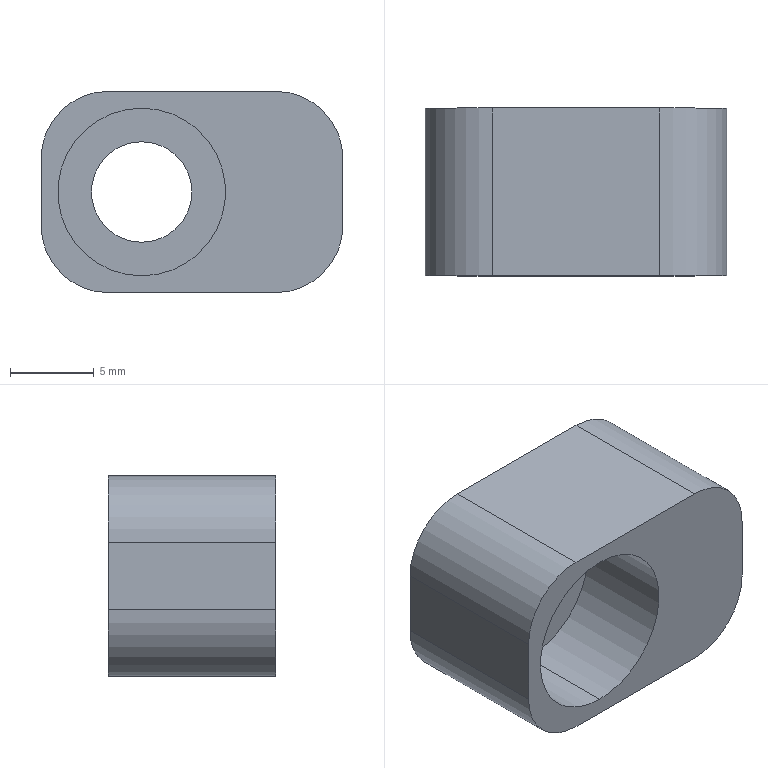Part | STEP file | 1 solid | 15 faces | box 18 x 10 x 12 mm | volume 1438 mm3 | cylinder 8 | plane 7 | commonest cylinder face diameters 8 x4 6 x2 10 x2
STEP:
#1=CARTESIAN_POINT('',(0.,0.,0.));
#2=DIRECTION('',(0.,0.,1.));
#3=DIRECTION('',(1.,0.,0.));
#4=AXIS2_PLACEMENT_3D('',#1,#2,#3);
#5=CARTESIAN_POINT('',(-138.148,-44.,136.665));
#6=VERTEX_POINT('',#5);
#7=CARTESIAN_POINT('',(-138.148,-40.,136.665));
#8=VERTEX_POINT('',#7);
#9=CARTESIAN_POINT('',(-138.148,-50.,136.665));
#10=DIRECTION('',(0.,1.,0.));
#11=VECTOR('',#10,1.);
#12=LINE('',#9,#11);
#13=CARTESIAN_POINT('',(-138.148,-50.,133.665));
#14=DIRECTION('',(0.,1.,0.));
#15=DIRECTION('',(0.,0.,1.));
#16=AXIS2_PLACEMENT_3D('',#13,#14,#15);
#17=CYLINDRICAL_SURFACE('',#16,3.);
#18=CARTESIAN_POINT('',(6.283,0.));
#19=DIRECTION('',(0.,1.));
#20=VECTOR('',#19,1.);
#21=LINE('',#18,#20);
#22=(GEOMETRIC_REPRESENTATION_CONTEXT(2)PARAMETRIC_REPRESENTATION_CONTEXT()REPRESENTATION_CONTEXT('',''));
#23=DEFINITIONAL_REPRESENTATION('',(#21),#22);
#24=PCURVE('',#17,#23);
#25=CARTESIAN_POINT('',(-138.148,-50.,133.665));
#26=DIRECTION('',(0.,1.,0.));
#27=DIRECTION('',(0.,0.,1.));
#28=AXIS2_PLACEMENT_3D('',#25,#26,#27);
#29=CYLINDRICAL_SURFACE('',#28,3.);
#30=CARTESIAN_POINT('',(0.,0.));
#31=DIRECTION('',(0.,1.));
#32=VECTOR('',#31,1.);
#33=LINE('',#30,#32);
#34=(GEOMETRIC_REPRESENTATION_CONTEXT(2)PARAMETRIC_REPRESENTATION_CONTEXT()REPRESENTATION_CONTEXT('',''));
#35=DEFINITIONAL_REPRESENTATION('',(#33),#34);
#36=PCURVE('',#29,#35);
#37=SURFACE_CURVE('',#12,(#24,#36),.PCURVE_S1.);
#38=EDGE_CURVE('',#6,#8,#37,.T.);
#39=ORIENTED_EDGE('',*,*,#38,.T.);
#40=CARTESIAN_POINT('',(-138.148,-40.,130.665));
#41=VERTEX_POINT('',#40);
#42=CARTESIAN_POINT('',(-138.148,-40.,133.665));
#43=DIRECTION('',(0.,-1.,0.));
#44=DIRECTION('',(0.,0.,-1.));
#45=AXIS2_PLACEMENT_3D('',#42,#43,#44);
#46=CIRCLE('',#45,3.);
#47=CARTESIAN_POINT('',(9.425,10.));
#48=DIRECTION('',(-1.,0.));
#49=VECTOR('',#48,1.);
#50=LINE('',#47,#49);
#51=(GEOMETRIC_REPRESENTATION_CONTEXT(2)PARAMETRIC_REPRESENTATION_CONTEXT()REPRESENTATION_CONTEXT('',''));
#52=DEFINITIONAL_REPRESENTATION('',(#50),#51);
#53=PCURVE('',#17,#52);
#54=CARTESIAN_POINT('',(-137.898,-40.,133.665));
#55=DIRECTION('',(0.,-1.,0.));
#56=DIRECTION('',(0.,0.,-1.));
#57=AXIS2_PLACEMENT_3D('',#54,#55,#56);
#58=PLANE('',#57);
#59=CARTESIAN_POINT('',(0.,-0.25));
#60=DIRECTION('',(1.,0.));
#61=AXIS2_PLACEMENT_2D('',#59,#60);
#62=CIRCLE('',#61,3.);
#63=(GEOMETRIC_REPRESENTATION_CONTEXT(2)PARAMETRIC_REPRESENTATION_CONTEXT()REPRESENTATION_CONTEXT('',''));
#64=DEFINITIONAL_REPRESENTATION('',(#62),#63);
#65=PCURVE('',#58,#64);
#66=SURFACE_CURVE('',#46,(#53,#65),.PCURVE_S1.);
#67=EDGE_CURVE('',#8,#41,#66,.T.);
#68=ORIENTED_EDGE('',*,*,#67,.T.);
#69=CARTESIAN_POINT('',(-138.148,-44.,130.665));
#70=VERTEX_POINT('',#69);
#71=CARTESIAN_POINT('',(-138.148,-50.,130.665));
#72=DIRECTION('',(0.,1.,0.));
#73=VECTOR('',#72,1.);
#74=LINE('',#71,#73);
#75=CARTESIAN_POINT('',(3.142,0.));
#76=DIRECTION('',(0.,1.));
#77=VECTOR('',#76,1.);
#78=LINE('',#75,#77);
#79=(GEOMETRIC_REPRESENTATION_CONTEXT(2)PARAMETRIC_REPRESENTATION_CONTEXT()REPRESENTATION_CONTEXT('',''));
#80=DEFINITIONAL_REPRESENTATION('',(#78),#79);
#81=PCURVE('',#17,#80);
#82=CARTESIAN_POINT('',(3.142,0.));
#83=DIRECTION('',(0.,1.));
#84=VECTOR('',#83,1.);
#85=LINE('',#82,#84);
#86=(GEOMETRIC_REPRESENTATION_CONTEXT(2)PARAMETRIC_REPRESENTATION_CONTEXT()REPRESENTATION_CONTEXT('',''));
#87=DEFINITIONAL_REPRESENTATION('',(#85),#86);
#88=PCURVE('',#29,#87);
#89=SURFACE_CURVE('',#74,(#81,#88),.PCURVE_S1.);
#90=EDGE_CURVE('',#70,#41,#89,.T.);
#91=ORIENTED_EDGE('',*,*,#90,.F.);
#92=CARTESIAN_POINT('',(-138.148,-44.,133.665));
#93=DIRECTION('',(0.,1.,0.));
#94=DIRECTION('',(0.,0.,1.));
#95=AXIS2_PLACEMENT_3D('',#92,#93,#94);
#96=CIRCLE('',#95,3.);
#97=CARTESIAN_POINT('',(0.,6.));
#98=DIRECTION('',(1.,0.));
#99=VECTOR('',#98,1.);
#100=LINE('',#97,#99);
#101=(GEOMETRIC_REPRESENTATION_CONTEXT(2)PARAMETRIC_REPRESENTATION_CONTEXT()REPRESENTATION_CONTEXT('',''));
#102=DEFINITIONAL_REPRESENTATION('',(#100),#101);
#103=PCURVE('',#17,#102);
#104=CARTESIAN_POINT('',(-138.148,-44.,133.665));
#105=DIRECTION('',(0.,1.,0.));
#106=DIRECTION('',(0.,0.,1.));
#107=AXIS2_PLACEMENT_3D('',#104,#105,#106);
#108=PLANE('',#107);
#109=CARTESIAN_POINT('',(0.,0.));
#110=DIRECTION('',(1.,0.));
#111=AXIS2_PLACEMENT_2D('',#109,#110);
#112=CIRCLE('',#111,3.);
#113=(GEOMETRIC_REPRESENTATION_CONTEXT(2)PARAMETRIC_REPRESENTATION_CONTEXT()REPRESENTATION_CONTEXT('',''));
#114=DEFINITIONAL_REPRESENTATION('',(#112),#113);
#115=PCURVE('',#108,#114);
#116=SURFACE_CURVE('',#96,(#103,#115),.PCURVE_S1.);
#117=EDGE_CURVE('',#70,#6,#116,.T.);
#118=ORIENTED_EDGE('',*,*,#117,.T.);
#119=EDGE_LOOP('',(#39,#68,#91,#118));
#120=FACE_BOUND('',#119,.F.);
#121=ADVANCED_FACE('',(#120),#17,.F.);
#122=CARTESIAN_POINT('',(-138.148,-50.,138.665));
#123=VERTEX_POINT('',#122);
#124=CARTESIAN_POINT('',(-138.148,-44.,138.665));
#125=VERTEX_POINT('',#124);
#126=CARTESIAN_POINT('',(-138.148,-50.,138.665));
#127=DIRECTION('',(0.,1.,0.));
#128=VECTOR('',#127,1.);
#129=LINE('',#126,#128);
#130=CARTESIAN_POINT('',(-138.148,-50.,133.665));
#131=DIRECTION('',(0.,1.,0.));
#132=DIRECTION('',(0.,0.,1.));
#133=AXIS2_PLACEMENT_3D('',#130,#131,#132);
#134=CYLINDRICAL_SURFACE('',#133,5.);
#135=CARTESIAN_POINT('',(6.283,0.));
#136=DIRECTION('',(0.,1.));
#137=VECTOR('',#136,1.);
#138=LINE('',#135,#137);
#139=(GEOMETRIC_REPRESENTATION_CONTEXT(2)PARAMETRIC_REPRESENTATION_CONTEXT()REPRESENTATION_CONTEXT('',''));
#140=DEFINITIONAL_REPRESENTATION('',(#138),#139);
#141=PCURVE('',#134,#140);
#142=CARTESIAN_POINT('',(-138.148,-50.,133.665));
#143=DIRECTION('',(0.,1.,0.));
#144=DIRECTION('',(0.,0.,1.));
#145=AXIS2_PLACEMENT_3D('',#142,#143,#144);
#146=CYLINDRICAL_SURFACE('',#145,5.);
#147=CARTESIAN_POINT('',(0.,0.));
#148=DIRECTION('',(0.,1.));
#149=VECTOR('',#148,1.);
#150=LINE('',#147,#149);
#151=(GEOMETRIC_REPRESENTATION_CONTEXT(2)PARAMETRIC_REPRESENTATION_CONTEXT()REPRESENTATION_CONTEXT('',''));
#152=DEFINITIONAL_REPRESENTATION('',(#150),#151);
#153=PCURVE('',#146,#152);
#154=SURFACE_CURVE('',#129,(#141,#153),.PCURVE_S1.);
#155=EDGE_CURVE('',#123,#125,#154,.T.);
#156=ORIENTED_EDGE('',*,*,#155,.T.);
#157=CARTESIAN_POINT('',(-138.148,-44.,128.665));
#158=VERTEX_POINT('',#157);
#159=CARTESIAN_POINT('',(-138.148,-44.,133.665));
#160=DIRECTION('',(0.,-1.,0.));
#161=DIRECTION('',(0.,0.,-1.));
#162=AXIS2_PLACEMENT_3D('',#159,#160,#161);
#163=CIRCLE('',#162,5.);
#164=CARTESIAN_POINT('',(9.425,6.));
#165=DIRECTION('',(-1.,0.));
#166=VECTOR('',#165,1.);
#167=LINE('',#164,#166);
#168=(GEOMETRIC_REPRESENTATION_CONTEXT(2)PARAMETRIC_REPRESENTATION_CONTEXT()REPRESENTATION_CONTEXT('',''));
#169=DEFINITIONAL_REPRESENTATION('',(#167),#168);
#170=PCURVE('',#134,#169);
#171=CARTESIAN_POINT('',(-5.,0.));
#172=CARTESIAN_POINT('',(-5.,8.66));
#173=CARTESIAN_POINT('',(2.5,4.33));
#174=CARTESIAN_POINT('',(10.,0.));
#175=CARTESIAN_POINT('',(2.5,-4.33));
#176=CARTESIAN_POINT('',(-5.,-8.66));
#177=CARTESIAN_POINT('',(-5.,0.));
#178=(BOUNDED_CURVE()B_SPLINE_CURVE(2,(#171,#172,#173,#174,#175,#176,#177),.UNSPECIFIED.,.T.,.F.)B_SPLINE_CURVE_WITH_KNOTS((1,2,2,2,2,1),(-2.094,0.,2.094,4.189,6.283,8.378),.UNSPECIFIED.)CURVE()GEOMETRIC_REPRESENTATION_ITEM()RATIONAL_B_SPLINE_CURVE((1.,0.5,1.,0.5,1.,0.5,1.))REPRESENTATION_ITEM(''));
#179=(GEOMETRIC_REPRESENTATION_CONTEXT(2)PARAMETRIC_REPRESENTATION_CONTEXT()REPRESENTATION_CONTEXT('',''));
#180=DEFINITIONAL_REPRESENTATION('',(#178),#179);
#181=PCURVE('',#108,#180);
#182=SURFACE_CURVE('',#163,(#170,#181),.PCURVE_S1.);
#183=EDGE_CURVE('',#125,#158,#182,.T.);
#184=ORIENTED_EDGE('',*,*,#183,.T.);
#185=CARTESIAN_POINT('',(-138.148,-50.,128.665));
#186=VERTEX_POINT('',#185);
#187=CARTESIAN_POINT('',(-138.148,-50.,128.665));
#188=DIRECTION('',(0.,1.,0.));
#189=VECTOR('',#188,1.);
#190=LINE('',#187,#189);
#191=CARTESIAN_POINT('',(3.142,0.));
#192=DIRECTION('',(0.,1.));
#193=VECTOR('',#192,1.);
#194=LINE('',#191,#193);
#195=(GEOMETRIC_REPRESENTATION_CONTEXT(2)PARAMETRIC_REPRESENTATION_CONTEXT()REPRESENTATION_CONTEXT('',''));
#196=DEFINITIONAL_REPRESENTATION('',(#194),#195);
#197=PCURVE('',#134,#196);
#198=CARTESIAN_POINT('',(3.142,0.));
#199=DIRECTION('',(0.,1.));
#200=VECTOR('',#199,1.);
#201=LINE('',#198,#200);
#202=(GEOMETRIC_REPRESENTATION_CONTEXT(2)PARAMETRIC_REPRESENTATION_CONTEXT()REPRESENTATION_CONTEXT('',''));
#203=DEFINITIONAL_REPRESENTATION('',(#201),#202);
#204=PCURVE('',#146,#203);
#205=SURFACE_CURVE('',#190,(#197,#204),.PCURVE_S1.);
#206=EDGE_CURVE('',#186,#158,#205,.T.);
#207=ORIENTED_EDGE('',*,*,#206,.F.);
#208=CARTESIAN_POINT('',(-138.148,-50.,133.665));
#209=DIRECTION('',(0.,1.,0.));
#210=DIRECTION('',(0.,0.,1.));
#211=AXIS2_PLACEMENT_3D('',#208,#209,#210);
#212=CIRCLE('',#211,5.);
#213=CARTESIAN_POINT('',(0.,0.));
#214=DIRECTION('',(1.,0.));
#215=VECTOR('',#214,1.);
#216=LINE('',#213,#215);
#217=(GEOMETRIC_REPRESENTATION_CONTEXT(2)PARAMETRIC_REPRESENTATION_CONTEXT()REPRESENTATION_CONTEXT('',''));
#218=DEFINITIONAL_REPRESENTATION('',(#216),#217);
#219=PCURVE('',#134,#218);
#220=CARTESIAN_POINT('',(-133.148,-50.,130.165));
#221=DIRECTION('',(0.,-1.,0.));
#222=DIRECTION('',(0.,0.,-1.));
#223=AXIS2_PLACEMENT_3D('',#220,#221,#222);
#224=PLANE('',#223);
#225=CARTESIAN_POINT('',(-8.5,-5.));
#226=CARTESIAN_POINT('',(-8.5,3.66));
#227=CARTESIAN_POINT('',(-1.,-0.6699));
#228=CARTESIAN_POINT('',(6.5,-5.));
#229=CARTESIAN_POINT('',(-1.,-9.33));
#230=CARTESIAN_POINT('',(-8.5,-13.66));
#231=CARTESIAN_POINT('',(-8.5,-5.));
#232=(BOUNDED_CURVE()B_SPLINE_CURVE(2,(#225,#226,#227,#228,#229,#230,#231),.UNSPECIFIED.,.T.,.F.)B_SPLINE_CURVE_WITH_KNOTS((1,2,2,2,2,1),(-2.094,0.,2.094,4.189,6.283,8.378),.UNSPECIFIED.)CURVE()GEOMETRIC_REPRESENTATION_ITEM()RATIONAL_B_SPLINE_CURVE((1.,0.5,1.,0.5,1.,0.5,1.))REPRESENTATION_ITEM(''));
#233=(GEOMETRIC_REPRESENTATION_CONTEXT(2)PARAMETRIC_REPRESENTATION_CONTEXT()REPRESENTATION_CONTEXT('',''));
#234=DEFINITIONAL_REPRESENTATION('',(#232),#233);
#235=PCURVE('',#224,#234);
#236=SURFACE_CURVE('',#212,(#219,#235),.PCURVE_S1.);
#237=EDGE_CURVE('',#186,#123,#236,.T.);
#238=ORIENTED_EDGE('',*,*,#237,.T.);
#239=EDGE_LOOP('',(#156,#184,#207,#238));
#240=FACE_BOUND('',#239,.F.);
#241=ADVANCED_FACE('',(#240),#134,.F.);
#242=CARTESIAN_POINT('',(-130.148,-50.,139.665));
#243=VERTEX_POINT('',#242);
#244=CARTESIAN_POINT('',(-140.148,-50.,139.665));
#245=VERTEX_POINT('',#244);
#246=CARTESIAN_POINT('',(-133.148,-50.,139.665));
#247=DIRECTION('',(-1.,0.,0.));
#248=VECTOR('',#247,1.);
#249=LINE('',#246,#248);
#250=CARTESIAN_POINT('',(-133.148,-43.,139.665));
#251=DIRECTION('',(0.,0.,1.));
#252=DIRECTION('',(1.,0.,0.));
#253=AXIS2_PLACEMENT_3D('',#250,#251,#252);
#254=PLANE('',#253);
#255=CARTESIAN_POINT('',(0.,-7.));
#256=DIRECTION('',(-1.,0.));
#257=VECTOR('',#256,1.);
#258=LINE('',#255,#257);
#259=(GEOMETRIC_REPRESENTATION_CONTEXT(2)PARAMETRIC_REPRESENTATION_CONTEXT()REPRESENTATION_CONTEXT('',''));
#260=DEFINITIONAL_REPRESENTATION('',(#258),#259);
#261=PCURVE('',#254,#260);
#262=CARTESIAN_POINT('',(-9.5,0.));
#263=DIRECTION('',(0.,-1.));
#264=VECTOR('',#263,1.);
#265=LINE('',#262,#264);
#266=(GEOMETRIC_REPRESENTATION_CONTEXT(2)PARAMETRIC_REPRESENTATION_CONTEXT()REPRESENTATION_CONTEXT('',''));
#267=DEFINITIONAL_REPRESENTATION('',(#265),#266);
#268=PCURVE('',#224,#267);
#269=SURFACE_CURVE('',#249,(#261,#268),.PCURVE_S1.);
#270=EDGE_CURVE('',#243,#245,#269,.T.);
#271=ORIENTED_EDGE('',*,*,#270,.F.);
#272=CARTESIAN_POINT('',(-130.148,-40.,139.665));
#273=VERTEX_POINT('',#272);
#274=CARTESIAN_POINT('',(-130.148,-43.,139.665));
#275=DIRECTION('',(0.,1.,0.));
#276=VECTOR('',#275,1.);
#277=LINE('',#274,#276);
#278=CARTESIAN_POINT('',(3.,0.));
#279=DIRECTION('',(0.,1.));
#280=VECTOR('',#279,1.);
#281=LINE('',#278,#280);
#282=(GEOMETRIC_REPRESENTATION_CONTEXT(2)PARAMETRIC_REPRESENTATION_CONTEXT()REPRESENTATION_CONTEXT('',''));
#283=DEFINITIONAL_REPRESENTATION('',(#281),#282);
#284=PCURVE('',#254,#283);
#285=CARTESIAN_POINT('',(-130.148,-45.,135.665));
#286=DIRECTION('',(0.,-1.,0.));
#287=DIRECTION('',(0.,0.,-1.));
#288=AXIS2_PLACEMENT_3D('',#285,#286,#287);
#289=CYLINDRICAL_SURFACE('',#288,4.);
#290=CARTESIAN_POINT('',(3.142,-2.));
#291=DIRECTION('',(0.,-1.));
#292=VECTOR('',#291,1.);
#293=LINE('',#290,#292);
#294=(GEOMETRIC_REPRESENTATION_CONTEXT(2)PARAMETRIC_REPRESENTATION_CONTEXT()REPRESENTATION_CONTEXT('',''));
#295=DEFINITIONAL_REPRESENTATION('',(#293),#294);
#296=PCURVE('',#289,#295);
#297=SURFACE_CURVE('',#277,(#284,#296),.PCURVE_S1.);
#298=EDGE_CURVE('',#243,#273,#297,.T.);
#299=ORIENTED_EDGE('',*,*,#298,.T.);
#300=CARTESIAN_POINT('',(-140.148,-40.,139.665));
#301=VERTEX_POINT('',#300);
#302=CARTESIAN_POINT('',(-133.148,-40.,139.665));
#303=DIRECTION('',(1.,0.,0.));
#304=VECTOR('',#303,1.);
#305=LINE('',#302,#304);
#306=CARTESIAN_POINT('',(0.,3.));
#307=DIRECTION('',(1.,0.));
#308=VECTOR('',#307,1.);
#309=LINE('',#306,#308);
#310=(GEOMETRIC_REPRESENTATION_CONTEXT(2)PARAMETRIC_REPRESENTATION_CONTEXT()REPRESENTATION_CONTEXT('',''));
#311=DEFINITIONAL_REPRESENTATION('',(#309),#310);
#312=PCURVE('',#254,#311);
#313=CARTESIAN_POINT('',(-6.,4.75));
#314=DIRECTION('',(0.,1.));
#315=VECTOR('',#314,1.);
#316=LINE('',#313,#315);
#317=(GEOMETRIC_REPRESENTATION_CONTEXT(2)PARAMETRIC_REPRESENTATION_CONTEXT()REPRESENTATION_CONTEXT('',''));
#318=DEFINITIONAL_REPRESENTATION('',(#316),#317);
#319=PCURVE('',#58,#318);
#320=SURFACE_CURVE('',#305,(#312,#319),.PCURVE_S1.);
#321=EDGE_CURVE('',#301,#273,#320,.T.);
#322=ORIENTED_EDGE('',*,*,#321,.F.);
#323=CARTESIAN_POINT('',(-140.148,-43.,139.665));
#324=DIRECTION('',(0.,-1.,0.));
#325=VECTOR('',#324,1.);
#326=LINE('',#323,#325);
#327=CARTESIAN_POINT('',(-7.,0.));
#328=DIRECTION('',(0.,-1.));
#329=VECTOR('',#328,1.);
#330=LINE('',#327,#329);
#331=(GEOMETRIC_REPRESENTATION_CONTEXT(2)PARAMETRIC_REPRESENTATION_CONTEXT()REPRESENTATION_CONTEXT('',''));
#332=DEFINITIONAL_REPRESENTATION('',(#330),#331);
#333=PCURVE('',#254,#332);
#334=CARTESIAN_POINT('',(-140.148,-43.,135.665));
#335=DIRECTION('',(0.,1.,0.));
#336=DIRECTION('',(0.,0.,1.));
#337=AXIS2_PLACEMENT_3D('',#334,#335,#336);
#338=CYLINDRICAL_SURFACE('',#337,4.);
#339=CARTESIAN_POINT('',(6.283,0.));
#340=DIRECTION('',(0.,-1.));
#341=VECTOR('',#340,1.);
#342=LINE('',#339,#341);
#343=(GEOMETRIC_REPRESENTATION_CONTEXT(2)PARAMETRIC_REPRESENTATION_CONTEXT()REPRESENTATION_CONTEXT('',''));
#344=DEFINITIONAL_REPRESENTATION('',(#342),#343);
#345=PCURVE('',#338,#344);
#346=SURFACE_CURVE('',#326,(#333,#345),.PCURVE_S1.);
#347=EDGE_CURVE('',#301,#245,#346,.T.);
#348=ORIENTED_EDGE('',*,*,#347,.T.);
#349=EDGE_LOOP('',(#271,#299,#322,#348));
#350=FACE_BOUND('',#349,.T.);
#351=ADVANCED_FACE('',(#350),#254,.T.);
#352=CARTESIAN_POINT('',(-138.148,-50.,133.665));
#353=DIRECTION('',(0.,1.,0.));
#354=DIRECTION('',(0.,0.,1.));
#355=AXIS2_PLACEMENT_3D('',#352,#353,#354);
#356=CIRCLE('',#355,5.);
#357=CARTESIAN_POINT('',(-8.5,-5.));
#358=CARTESIAN_POINT('',(-8.5,3.66));
#359=CARTESIAN_POINT('',(-1.,-0.6699));
#360=CARTESIAN_POINT('',(6.5,-5.));
#361=CARTESIAN_POINT('',(-1.,-9.33));
#362=CARTESIAN_POINT('',(-8.5,-13.66));
#363=CARTESIAN_POINT('',(-8.5,-5.));
#364=(BOUNDED_CURVE()B_SPLINE_CURVE(2,(#357,#358,#359,#360,#361,#362,#363),.UNSPECIFIED.,.T.,.F.)B_SPLINE_CURVE_WITH_KNOTS((1,2,2,2,2,1),(-2.094,0.,2.094,4.189,6.283,8.378),.UNSPECIFIED.)CURVE()GEOMETRIC_REPRESENTATION_ITEM()RATIONAL_B_SPLINE_CURVE((1.,0.5,1.,0.5,1.,0.5,1.))REPRESENTATION_ITEM(''));
#365=(GEOMETRIC_REPRESENTATION_CONTEXT(2)PARAMETRIC_REPRESENTATION_CONTEXT()REPRESENTATION_CONTEXT('',''));
#366=DEFINITIONAL_REPRESENTATION('',(#364),#365);
#367=PCURVE('',#224,#366);
#368=CARTESIAN_POINT('',(0.,0.));
#369=DIRECTION('',(1.,0.));
#370=VECTOR('',#369,1.);
#371=LINE('',#368,#370);
#372=(GEOMETRIC_REPRESENTATION_CONTEXT(2)PARAMETRIC_REPRESENTATION_CONTEXT()REPRESENTATION_CONTEXT('',''));
#373=DEFINITIONAL_REPRESENTATION('',(#371),#372);
#374=PCURVE('',#146,#373);
#375=SURFACE_CURVE('',#356,(#367,#374),.PCURVE_S1.);
#376=EDGE_CURVE('',#123,#186,#375,.T.);
#377=ORIENTED_EDGE('',*,*,#376,.T.);
#378=ORIENTED_EDGE('',*,*,#237,.T.);
#379=EDGE_LOOP('',(#377,#378));
#380=FACE_BOUND('',#379,.T.);
#381=CARTESIAN_POINT('',(-126.147,-50.,131.665));
#382=VERTEX_POINT('',#381);
#383=CARTESIAN_POINT('',(-126.147,-50.,135.665));
#384=VERTEX_POINT('',#383);
#385=CARTESIAN_POINT('',(-126.147,-50.,127.665));
#386=DIRECTION('',(0.,0.,1.));
#387=VECTOR('',#386,1.);
#388=LINE('',#385,#387);
#389=CARTESIAN_POINT('',(2.5,7.));
#390=DIRECTION('',(-1.,0.));
#391=VECTOR('',#390,1.);
#392=LINE('',#389,#391);
#393=(GEOMETRIC_REPRESENTATION_CONTEXT(2)PARAMETRIC_REPRESENTATION_CONTEXT()REPRESENTATION_CONTEXT('',''));
#394=DEFINITIONAL_REPRESENTATION('',(#392),#393);
#395=PCURVE('',#224,#394);
#396=CARTESIAN_POINT('',(-126.147,-45.,127.665));
#397=DIRECTION('',(1.,0.,0.));
#398=DIRECTION('',(0.,0.,-1.));
#399=AXIS2_PLACEMENT_3D('',#396,#397,#398);
#400=PLANE('',#399);
#401=CARTESIAN_POINT('',(0.,-5.));
#402=DIRECTION('',(-1.,0.));
#403=VECTOR('',#402,1.);
#404=LINE('',#401,#403);
#405=(GEOMETRIC_REPRESENTATION_CONTEXT(2)PARAMETRIC_REPRESENTATION_CONTEXT()REPRESENTATION_CONTEXT('',''));
#406=DEFINITIONAL_REPRESENTATION('',(#404),#405);
#407=PCURVE('',#400,#406);
#408=SURFACE_CURVE('',#388,(#395,#407),.PCURVE_S1.);
#409=EDGE_CURVE('',#382,#384,#408,.T.);
#410=ORIENTED_EDGE('',*,*,#409,.T.);
#411=CARTESIAN_POINT('',(-130.148,-50.,135.665));
#412=DIRECTION('',(0.,-1.,0.));
#413=DIRECTION('',(0.,0.,-1.));
#414=AXIS2_PLACEMENT_3D('',#411,#412,#413);
#415=CIRCLE('',#414,4.);
#416=CARTESIAN_POINT('',(-5.5,3.));
#417=DIRECTION('',(1.,0.));
#418=AXIS2_PLACEMENT_2D('',#416,#417);
#419=CIRCLE('',#418,4.);
#420=(GEOMETRIC_REPRESENTATION_CONTEXT(2)PARAMETRIC_REPRESENTATION_CONTEXT()REPRESENTATION_CONTEXT('',''));
#421=DEFINITIONAL_REPRESENTATION('',(#419),#420);
#422=PCURVE('',#224,#421);
#423=CARTESIAN_POINT('',(0.,5.));
#424=DIRECTION('',(1.,0.));
#425=VECTOR('',#424,1.);
#426=LINE('',#423,#425);
#427=(GEOMETRIC_REPRESENTATION_CONTEXT(2)PARAMETRIC_REPRESENTATION_CONTEXT()REPRESENTATION_CONTEXT('',''));
#428=DEFINITIONAL_REPRESENTATION('',(#426),#427);
#429=PCURVE('',#289,#428);
#430=SURFACE_CURVE('',#415,(#422,#429),.PCURVE_S1.);
#431=EDGE_CURVE('',#384,#243,#430,.T.);
#432=ORIENTED_EDGE('',*,*,#431,.T.);
#433=ORIENTED_EDGE('',*,*,#270,.T.);
#434=CARTESIAN_POINT('',(-144.148,-50.,135.665));
#435=VERTEX_POINT('',#434);
#436=CARTESIAN_POINT('',(-140.148,-50.,135.665));
#437=DIRECTION('',(0.,-1.,0.));
#438=DIRECTION('',(0.,0.,-1.));
#439=AXIS2_PLACEMENT_3D('',#436,#437,#438);
#440=CIRCLE('',#439,4.);
#441=CARTESIAN_POINT('',(-5.5,-7.));
#442=DIRECTION('',(1.,0.));
#443=AXIS2_PLACEMENT_2D('',#441,#442);
#444=CIRCLE('',#443,4.);
#445=(GEOMETRIC_REPRESENTATION_CONTEXT(2)PARAMETRIC_REPRESENTATION_CONTEXT()REPRESENTATION_CONTEXT('',''));
#446=DEFINITIONAL_REPRESENTATION('',(#444),#445);
#447=PCURVE('',#224,#446);
#448=CARTESIAN_POINT('',(9.425,-7.));
#449=DIRECTION('',(-1.,0.));
#450=VECTOR('',#449,1.);
#451=LINE('',#448,#450);
#452=(GEOMETRIC_REPRESENTATION_CONTEXT(2)PARAMETRIC_REPRESENTATION_CONTEXT()REPRESENTATION_CONTEXT('',''));
#453=DEFINITIONAL_REPRESENTATION('',(#451),#452);
#454=PCURVE('',#338,#453);
#455=SURFACE_CURVE('',#440,(#447,#454),.PCURVE_S1.);
#456=EDGE_CURVE('',#245,#435,#455,.T.);
#457=ORIENTED_EDGE('',*,*,#456,.T.);
#458=CARTESIAN_POINT('',(-144.148,-50.,131.665));
#459=VERTEX_POINT('',#458);
#460=CARTESIAN_POINT('',(-144.148,-50.,130.165));
#461=DIRECTION('',(0.,0.,1.));
#462=VECTOR('',#461,1.);
#463=LINE('',#460,#462);
#464=CARTESIAN_POINT('',(0.,-11.));
#465=DIRECTION('',(-1.,0.));
#466=VECTOR('',#465,1.);
#467=LINE('',#464,#466);
#468=(GEOMETRIC_REPRESENTATION_CONTEXT(2)PARAMETRIC_REPRESENTATION_CONTEXT()REPRESENTATION_CONTEXT('',''));
#469=DEFINITIONAL_REPRESENTATION('',(#467),#468);
#470=PCURVE('',#224,#469);
#471=CARTESIAN_POINT('',(-144.148,-43.,130.165));
#472=DIRECTION('',(-1.,0.,0.));
#473=DIRECTION('',(0.,0.,1.));
#474=AXIS2_PLACEMENT_3D('',#471,#472,#473);
#475=PLANE('',#474);
#476=CARTESIAN_POINT('',(0.,-7.));
#477=DIRECTION('',(1.,0.));
#478=VECTOR('',#477,1.);
#479=LINE('',#476,#478);
#480=(GEOMETRIC_REPRESENTATION_CONTEXT(2)PARAMETRIC_REPRESENTATION_CONTEXT()REPRESENTATION_CONTEXT('',''));
#481=DEFINITIONAL_REPRESENTATION('',(#479),#480);
#482=PCURVE('',#475,#481);
#483=SURFACE_CURVE('',#463,(#470,#482),.PCURVE_S1.);
#484=EDGE_CURVE('',#459,#435,#483,.T.);
#485=ORIENTED_EDGE('',*,*,#484,.F.);
#486=CARTESIAN_POINT('',(-140.148,-50.,127.665));
#487=VERTEX_POINT('',#486);
#488=CARTESIAN_POINT('',(-140.148,-50.,131.665));
#489=DIRECTION('',(0.,-1.,0.));
#490=DIRECTION('',(0.,0.,-1.));
#491=AXIS2_PLACEMENT_3D('',#488,#489,#490);
#492=CIRCLE('',#491,4.);
#493=CARTESIAN_POINT('',(-1.5,-7.));
#494=DIRECTION('',(1.,0.));
#495=AXIS2_PLACEMENT_2D('',#493,#494);
#496=CIRCLE('',#495,4.);
#497=(GEOMETRIC_REPRESENTATION_CONTEXT(2)PARAMETRIC_REPRESENTATION_CONTEXT()REPRESENTATION_CONTEXT('',''));
#498=DEFINITIONAL_REPRESENTATION('',(#496),#497);
#499=PCURVE('',#224,#498);
#500=CARTESIAN_POINT('',(-140.148,-43.,131.665));
#501=DIRECTION('',(0.,-1.,0.));
#502=DIRECTION('',(0.,0.,-1.));
#503=AXIS2_PLACEMENT_3D('',#500,#501,#502);
#504=CYLINDRICAL_SURFACE('',#503,4.);
#505=CARTESIAN_POINT('',(0.,7.));
#506=DIRECTION('',(1.,0.));
#507=VECTOR('',#506,1.);
#508=LINE('',#505,#507);
#509=(GEOMETRIC_REPRESENTATION_CONTEXT(2)PARAMETRIC_REPRESENTATION_CONTEXT()REPRESENTATION_CONTEXT('',''));
#510=DEFINITIONAL_REPRESENTATION('',(#508),#509);
#511=PCURVE('',#504,#510);
#512=SURFACE_CURVE('',#492,(#499,#511),.PCURVE_S1.);
#513=EDGE_CURVE('',#459,#487,#512,.T.);
#514=ORIENTED_EDGE('',*,*,#513,.T.);
#515=CARTESIAN_POINT('',(-130.148,-50.,127.665));
#516=VERTEX_POINT('',#515);
#517=CARTESIAN_POINT('',(-133.148,-50.,127.665));
#518=DIRECTION('',(1.,0.,0.));
#519=VECTOR('',#518,1.);
#520=LINE('',#517,#519);
#521=CARTESIAN_POINT('',(2.5,0.));
#522=DIRECTION('',(0.,1.));
#523=VECTOR('',#522,1.);
#524=LINE('',#521,#523);
#525=(GEOMETRIC_REPRESENTATION_CONTEXT(2)PARAMETRIC_REPRESENTATION_CONTEXT()REPRESENTATION_CONTEXT('',''));
#526=DEFINITIONAL_REPRESENTATION('',(#524),#525);
#527=PCURVE('',#224,#526);
#528=CARTESIAN_POINT('',(-133.148,-43.,127.665));
#529=DIRECTION('',(0.,0.,-1.));
#530=DIRECTION('',(-1.,0.,0.));
#531=AXIS2_PLACEMENT_3D('',#528,#529,#530);
#532=PLANE('',#531);
#533=CARTESIAN_POINT('',(0.,-7.));
#534=DIRECTION('',(-1.,0.));
#535=VECTOR('',#534,1.);
#536=LINE('',#533,#535);
#537=(GEOMETRIC_REPRESENTATION_CONTEXT(2)PARAMETRIC_REPRESENTATION_CONTEXT()REPRESENTATION_CONTEXT('',''));
#538=DEFINITIONAL_REPRESENTATION('',(#536),#537);
#539=PCURVE('',#532,#538);
#540=SURFACE_CURVE('',#520,(#527,#539),.PCURVE_S1.);
#541=EDGE_CURVE('',#487,#516,#540,.T.);
#542=ORIENTED_EDGE('',*,*,#541,.T.);
#543=CARTESIAN_POINT('',(-130.148,-50.,131.665));
#544=DIRECTION('',(0.,-1.,0.));
#545=DIRECTION('',(0.,0.,-1.));
#546=AXIS2_PLACEMENT_3D('',#543,#544,#545);
#547=CIRCLE('',#546,4.);
#548=CARTESIAN_POINT('',(-1.5,3.));
#549=DIRECTION('',(1.,0.));
#550=AXIS2_PLACEMENT_2D('',#548,#549);
#551=CIRCLE('',#550,4.);
#552=(GEOMETRIC_REPRESENTATION_CONTEXT(2)PARAMETRIC_REPRESENTATION_CONTEXT()REPRESENTATION_CONTEXT('',''));
#553=DEFINITIONAL_REPRESENTATION('',(#551),#552);
#554=PCURVE('',#224,#553);
#555=CARTESIAN_POINT('',(-130.148,-45.,131.665));
#556=DIRECTION('',(0.,1.,0.));
#557=DIRECTION('',(0.,0.,1.));
#558=AXIS2_PLACEMENT_3D('',#555,#556,#557);
#559=CYLINDRICAL_SURFACE('',#558,4.);
#560=CARTESIAN_POINT('',(3.142,-5.));
#561=DIRECTION('',(-1.,0.));
#562=VECTOR('',#561,1.);
#563=LINE('',#560,#562);
#564=(GEOMETRIC_REPRESENTATION_CONTEXT(2)PARAMETRIC_REPRESENTATION_CONTEXT()REPRESENTATION_CONTEXT('',''));
#565=DEFINITIONAL_REPRESENTATION('',(#563),#564);
#566=PCURVE('',#559,#565);
#567=SURFACE_CURVE('',#547,(#554,#566),.PCURVE_S1.);
#568=EDGE_CURVE('',#516,#382,#567,.T.);
#569=ORIENTED_EDGE('',*,*,#568,.T.);
#570=EDGE_LOOP('',(#410,#432,#433,#457,#485,#514,#542,#569));
#571=FACE_BOUND('',#570,.T.);
#572=ADVANCED_FACE('',(#380,#571),#224,.T.);
#573=ORIENTED_EDGE('',*,*,#484,.T.);
#574=CARTESIAN_POINT('',(-144.148,-40.,135.665));
#575=VERTEX_POINT('',#574);
#576=CARTESIAN_POINT('',(-144.148,-43.,135.665));
#577=DIRECTION('',(0.,1.,0.));
#578=VECTOR('',#577,1.);
#579=LINE('',#576,#578);
#580=CARTESIAN_POINT('',(5.5,0.));
#581=DIRECTION('',(0.,1.));
#582=VECTOR('',#581,1.);
#583=LINE('',#580,#582);
#584=(GEOMETRIC_REPRESENTATION_CONTEXT(2)PARAMETRIC_REPRESENTATION_CONTEXT()REPRESENTATION_CONTEXT('',''));
#585=DEFINITIONAL_REPRESENTATION('',(#583),#584);
#586=PCURVE('',#475,#585);
#587=CARTESIAN_POINT('',(4.712,0.));
#588=DIRECTION('',(0.,1.));
#589=VECTOR('',#588,1.);
#590=LINE('',#587,#589);
#591=(GEOMETRIC_REPRESENTATION_CONTEXT(2)PARAMETRIC_REPRESENTATION_CONTEXT()REPRESENTATION_CONTEXT('',''));
#592=DEFINITIONAL_REPRESENTATION('',(#590),#591);
#593=PCURVE('',#338,#592);
#594=SURFACE_CURVE('',#579,(#586,#593),.PCURVE_S1.);
#595=EDGE_CURVE('',#435,#575,#594,.T.);
#596=ORIENTED_EDGE('',*,*,#595,.T.);
#597=CARTESIAN_POINT('',(-144.148,-40.,131.665));
#598=VERTEX_POINT('',#597);
#599=CARTESIAN_POINT('',(-144.148,-40.,130.165));
#600=DIRECTION('',(0.,0.,1.));
#601=VECTOR('',#600,1.);
#602=LINE('',#599,#601);
#603=CARTESIAN_POINT('',(0.,3.));
#604=DIRECTION('',(1.,0.));
#605=VECTOR('',#604,1.);
#606=LINE('',#603,#605);
#607=(GEOMETRIC_REPRESENTATION_CONTEXT(2)PARAMETRIC_REPRESENTATION_CONTEXT()REPRESENTATION_CONTEXT('',''));
#608=DEFINITIONAL_REPRESENTATION('',(#606),#607);
#609=PCURVE('',#475,#608);
#610=CARTESIAN_POINT('',(3.5,-6.25));
#611=DIRECTION('',(-1.,0.));
#612=VECTOR('',#611,1.);
#613=LINE('',#610,#612);
#614=(GEOMETRIC_REPRESENTATION_CONTEXT(2)PARAMETRIC_REPRESENTATION_CONTEXT()REPRESENTATION_CONTEXT('',''));
#615=DEFINITIONAL_REPRESENTATION('',(#613),#614);
#616=PCURVE('',#58,#615);
#617=SURFACE_CURVE('',#602,(#609,#616),.PCURVE_S1.);
#618=EDGE_CURVE('',#598,#575,#617,.T.);
#619=ORIENTED_EDGE('',*,*,#618,.F.);
#620=CARTESIAN_POINT('',(-144.148,-43.,131.665));
#621=DIRECTION('',(0.,-1.,0.));
#622=VECTOR('',#621,1.);
#623=LINE('',#620,#622);
#624=CARTESIAN_POINT('',(1.5,0.));
#625=DIRECTION('',(0.,-1.));
#626=VECTOR('',#625,1.);
#627=LINE('',#624,#626);
#628=(GEOMETRIC_REPRESENTATION_CONTEXT(2)PARAMETRIC_REPRESENTATION_CONTEXT()REPRESENTATION_CONTEXT('',''));
#629=DEFINITIONAL_REPRESENTATION('',(#627),#628);
#630=PCURVE('',#475,#629);
#631=CARTESIAN_POINT('',(4.712,0.));
#632=DIRECTION('',(0.,1.));
#633=VECTOR('',#632,1.);
#634=LINE('',#631,#633);
#635=(GEOMETRIC_REPRESENTATION_CONTEXT(2)PARAMETRIC_REPRESENTATION_CONTEXT()REPRESENTATION_CONTEXT('',''));
#636=DEFINITIONAL_REPRESENTATION('',(#634),#635);
#637=PCURVE('',#504,#636);
#638=SURFACE_CURVE('',#623,(#630,#637),.PCURVE_S1.);
#639=EDGE_CURVE('',#598,#459,#638,.T.);
#640=ORIENTED_EDGE('',*,*,#639,.T.);
#641=EDGE_LOOP('',(#573,#596,#619,#640));
#642=FACE_BOUND('',#641,.T.);
#643=ADVANCED_FACE('',(#642),#475,.T.);
#644=CARTESIAN_POINT('',(-130.148,-40.,127.665));
#645=VERTEX_POINT('',#644);
#646=CARTESIAN_POINT('',(-140.148,-40.,127.665));
#647=VERTEX_POINT('',#646);
#648=CARTESIAN_POINT('',(-133.148,-40.,127.665));
#649=DIRECTION('',(-1.,0.,0.));
#650=VECTOR('',#649,1.);
#651=LINE('',#648,#650);
#652=CARTESIAN_POINT('',(0.,3.));
#653=DIRECTION('',(1.,0.));
#654=VECTOR('',#653,1.);
#655=LINE('',#652,#654);
#656=(GEOMETRIC_REPRESENTATION_CONTEXT(2)PARAMETRIC_REPRESENTATION_CONTEXT()REPRESENTATION_CONTEXT('',''));
#657=DEFINITIONAL_REPRESENTATION('',(#655),#656);
#658=PCURVE('',#532,#657);
#659=CARTESIAN_POINT('',(6.,4.75));
#660=DIRECTION('',(0.,-1.));
#661=VECTOR('',#660,1.);
#662=LINE('',#659,#661);
#663=(GEOMETRIC_REPRESENTATION_CONTEXT(2)PARAMETRIC_REPRESENTATION_CONTEXT()REPRESENTATION_CONTEXT('',''));
#664=DEFINITIONAL_REPRESENTATION('',(#662),#663);
#665=PCURVE('',#58,#664);
#666=SURFACE_CURVE('',#651,(#658,#665),.PCURVE_S1.);
#667=EDGE_CURVE('',#645,#647,#666,.T.);
#668=ORIENTED_EDGE('',*,*,#667,.F.);
#669=CARTESIAN_POINT('',(-130.148,-43.,127.665));
#670=DIRECTION('',(0.,-1.,0.));
#671=VECTOR('',#670,1.);
#672=LINE('',#669,#671);
#673=CARTESIAN_POINT('',(-3.,0.));
#674=DIRECTION('',(0.,-1.));
#675=VECTOR('',#674,1.);
#676=LINE('',#673,#675);
#677=(GEOMETRIC_REPRESENTATION_CONTEXT(2)PARAMETRIC_REPRESENTATION_CONTEXT()REPRESENTATION_CONTEXT('',''));
#678=DEFINITIONAL_REPRESENTATION('',(#676),#677);
#679=PCURVE('',#532,#678);
#680=CARTESIAN_POINT('',(3.142,2.));
#681=DIRECTION('',(0.,-1.));
#682=VECTOR('',#681,1.);
#683=LINE('',#680,#682);
#684=(GEOMETRIC_REPRESENTATION_CONTEXT(2)PARAMETRIC_REPRESENTATION_CONTEXT()REPRESENTATION_CONTEXT('',''));
#685=DEFINITIONAL_REPRESENTATION('',(#683),#684);
#686=PCURVE('',#559,#685);
#687=SURFACE_CURVE('',#672,(#679,#686),.PCURVE_S1.);
#688=EDGE_CURVE('',#645,#516,#687,.T.);
#689=ORIENTED_EDGE('',*,*,#688,.T.);
#690=ORIENTED_EDGE('',*,*,#541,.F.);
#691=CARTESIAN_POINT('',(-140.148,-43.,127.665));
#692=DIRECTION('',(0.,1.,0.));
#693=VECTOR('',#692,1.);
#694=LINE('',#691,#693);
#695=CARTESIAN_POINT('',(7.,0.));
#696=DIRECTION('',(0.,1.));
#697=VECTOR('',#696,1.);
#698=LINE('',#695,#697);
#699=(GEOMETRIC_REPRESENTATION_CONTEXT(2)PARAMETRIC_REPRESENTATION_CONTEXT()REPRESENTATION_CONTEXT('',''));
#700=DEFINITIONAL_REPRESENTATION('',(#698),#699);
#701=PCURVE('',#532,#700);
#702=CARTESIAN_POINT('',(6.283,0.));
#703=DIRECTION('',(0.,-1.));
#704=VECTOR('',#703,1.);
#705=LINE('',#702,#704);
#706=(GEOMETRIC_REPRESENTATION_CONTEXT(2)PARAMETRIC_REPRESENTATION_CONTEXT()REPRESENTATION_CONTEXT('',''));
#707=DEFINITIONAL_REPRESENTATION('',(#705),#706);
#708=PCURVE('',#504,#707);
#709=SURFACE_CURVE('',#694,(#701,#708),.PCURVE_S1.);
#710=EDGE_CURVE('',#487,#647,#709,.T.);
#711=ORIENTED_EDGE('',*,*,#710,.T.);
#712=EDGE_LOOP('',(#668,#689,#690,#711));
#713=FACE_BOUND('',#712,.T.);
#714=ADVANCED_FACE('',(#713),#532,.T.);
#715=ORIENTED_EDGE('',*,*,#321,.T.);
#716=CARTESIAN_POINT('',(-126.147,-40.,135.665));
#717=VERTEX_POINT('',#716);
#718=CARTESIAN_POINT('',(-130.148,-40.,135.665));
#719=DIRECTION('',(0.,1.,0.));
#720=DIRECTION('',(0.,0.,-1.));
#721=AXIS2_PLACEMENT_3D('',#718,#719,#720);
#722=CIRCLE('',#721,4.);
#723=CARTESIAN_POINT('',(2.,7.75));
#724=CARTESIAN_POINT('',(2.,0.8218));
#725=CARTESIAN_POINT('',(-4.,4.286));
#726=CARTESIAN_POINT('',(-10.,7.75));
#727=CARTESIAN_POINT('',(-4.,11.214));
#728=CARTESIAN_POINT('',(2.,14.678));
#729=CARTESIAN_POINT('',(2.,7.75));
#730=(BOUNDED_CURVE()B_SPLINE_CURVE(2,(#723,#724,#725,#726,#727,#728,#729),.UNSPECIFIED.,.T.,.F.)B_SPLINE_CURVE_WITH_KNOTS((1,2,2,2,2,1),(-2.094,0.,2.094,4.189,6.283,8.378),.UNSPECIFIED.)CURVE()GEOMETRIC_REPRESENTATION_ITEM()RATIONAL_B_SPLINE_CURVE((1.,0.5,1.,0.5,1.,0.5,1.))REPRESENTATION_ITEM(''));
#731=(GEOMETRIC_REPRESENTATION_CONTEXT(2)PARAMETRIC_REPRESENTATION_CONTEXT()REPRESENTATION_CONTEXT('',''));
#732=DEFINITIONAL_REPRESENTATION('',(#730),#731);
#733=PCURVE('',#58,#732);
#734=CARTESIAN_POINT('',(6.283,-5.));
#735=DIRECTION('',(-1.,0.));
#736=VECTOR('',#735,1.);
#737=LINE('',#734,#736);
#738=(GEOMETRIC_REPRESENTATION_CONTEXT(2)PARAMETRIC_REPRESENTATION_CONTEXT()REPRESENTATION_CONTEXT('',''));
#739=DEFINITIONAL_REPRESENTATION('',(#737),#738);
#740=PCURVE('',#289,#739);
#741=SURFACE_CURVE('',#722,(#733,#740),.PCURVE_S1.);
#742=EDGE_CURVE('',#273,#717,#741,.T.);
#743=ORIENTED_EDGE('',*,*,#742,.T.);
#744=CARTESIAN_POINT('',(-126.147,-40.,131.665));
#745=VERTEX_POINT('',#744);
#746=CARTESIAN_POINT('',(-126.147,-40.,127.665));
#747=DIRECTION('',(0.,0.,1.));
#748=VECTOR('',#747,1.);
#749=LINE('',#746,#748);
#750=CARTESIAN_POINT('',(6.,11.75));
#751=DIRECTION('',(-1.,0.));
#752=VECTOR('',#751,1.);
#753=LINE('',#750,#752);
#754=(GEOMETRIC_REPRESENTATION_CONTEXT(2)PARAMETRIC_REPRESENTATION_CONTEXT()REPRESENTATION_CONTEXT('',''));
#755=DEFINITIONAL_REPRESENTATION('',(#753),#754);
#756=PCURVE('',#58,#755);
#757=CARTESIAN_POINT('',(0.,5.));
#758=DIRECTION('',(-1.,0.));
#759=VECTOR('',#758,1.);
#760=LINE('',#757,#759);
#761=(GEOMETRIC_REPRESENTATION_CONTEXT(2)PARAMETRIC_REPRESENTATION_CONTEXT()REPRESENTATION_CONTEXT('',''));
#762=DEFINITIONAL_REPRESENTATION('',(#760),#761);
#763=PCURVE('',#400,#762);
#764=SURFACE_CURVE('',#749,(#756,#763),.PCURVE_S1.);
#765=EDGE_CURVE('',#745,#717,#764,.T.);
#766=ORIENTED_EDGE('',*,*,#765,.F.);
#767=CARTESIAN_POINT('',(-130.148,-40.,131.665));
#768=DIRECTION('',(0.,1.,0.));
#769=DIRECTION('',(0.,0.,-1.));
#770=AXIS2_PLACEMENT_3D('',#767,#768,#769);
#771=CIRCLE('',#770,4.);
#772=CARTESIAN_POINT('',(6.,7.75));
#773=CARTESIAN_POINT('',(6.,0.8218));
#774=CARTESIAN_POINT('',(0.,4.286));
#775=CARTESIAN_POINT('',(-6.,7.75));
#776=CARTESIAN_POINT('',(0.,11.214));
#777=CARTESIAN_POINT('',(6.,14.678));
#778=CARTESIAN_POINT('',(6.,7.75));
#779=(BOUNDED_CURVE()B_SPLINE_CURVE(2,(#772,#773,#774,#775,#776,#777,#778),.UNSPECIFIED.,.T.,.F.)B_SPLINE_CURVE_WITH_KNOTS((1,2,2,2,2,1),(-2.094,0.,2.094,4.189,6.283,8.378),.UNSPECIFIED.)CURVE()GEOMETRIC_REPRESENTATION_ITEM()RATIONAL_B_SPLINE_CURVE((1.,0.5,1.,0.5,1.,0.5,1.))REPRESENTATION_ITEM(''));
#780=(GEOMETRIC_REPRESENTATION_CONTEXT(2)PARAMETRIC_REPRESENTATION_CONTEXT()REPRESENTATION_CONTEXT('',''));
#781=DEFINITIONAL_REPRESENTATION('',(#779),#780);
#782=PCURVE('',#58,#781);
#783=CARTESIAN_POINT('',(-3.142,5.));
#784=DIRECTION('',(1.,0.));
#785=VECTOR('',#784,1.);
#786=LINE('',#783,#785);
#787=(GEOMETRIC_REPRESENTATION_CONTEXT(2)PARAMETRIC_REPRESENTATION_CONTEXT()REPRESENTATION_CONTEXT('',''));
#788=DEFINITIONAL_REPRESENTATION('',(#786),#787);
#789=PCURVE('',#559,#788);
#790=SURFACE_CURVE('',#771,(#782,#789),.PCURVE_S1.);
#791=EDGE_CURVE('',#745,#645,#790,.T.);
#792=ORIENTED_EDGE('',*,*,#791,.T.);
#793=ORIENTED_EDGE('',*,*,#667,.T.);
#794=CARTESIAN_POINT('',(-140.148,-40.,131.665));
#795=DIRECTION('',(0.,1.,0.));
#796=DIRECTION('',(0.,0.,-1.));
#797=AXIS2_PLACEMENT_3D('',#794,#795,#796);
#798=CIRCLE('',#797,4.);
#799=CARTESIAN_POINT('',(6.,-2.25));
#800=CARTESIAN_POINT('',(6.,-9.178));
#801=CARTESIAN_POINT('',(0.,-5.714));
#802=CARTESIAN_POINT('',(-6.,-2.25));
#803=CARTESIAN_POINT('',(0.,1.214));
#804=CARTESIAN_POINT('',(6.,4.678));
#805=CARTESIAN_POINT('',(6.,-2.25));
#806=(BOUNDED_CURVE()B_SPLINE_CURVE(2,(#799,#800,#801,#802,#803,#804,#805),.UNSPECIFIED.,.T.,.F.)B_SPLINE_CURVE_WITH_KNOTS((1,2,2,2,2,1),(-2.094,0.,2.094,4.189,6.283,8.378),.UNSPECIFIED.)CURVE()GEOMETRIC_REPRESENTATION_ITEM()RATIONAL_B_SPLINE_CURVE((1.,0.5,1.,0.5,1.,0.5,1.))REPRESENTATION_ITEM(''));
#807=(GEOMETRIC_REPRESENTATION_CONTEXT(2)PARAMETRIC_REPRESENTATION_CONTEXT()REPRESENTATION_CONTEXT('',''));
#808=DEFINITIONAL_REPRESENTATION('',(#806),#807);
#809=PCURVE('',#58,#808);
#810=CARTESIAN_POINT('',(6.283,-3.));
#811=DIRECTION('',(-1.,0.));
#812=VECTOR('',#811,1.);
#813=LINE('',#810,#812);
#814=(GEOMETRIC_REPRESENTATION_CONTEXT(2)PARAMETRIC_REPRESENTATION_CONTEXT()REPRESENTATION_CONTEXT('',''));
#815=DEFINITIONAL_REPRESENTATION('',(#813),#814);
#816=PCURVE('',#504,#815);
#817=SURFACE_CURVE('',#798,(#809,#816),.PCURVE_S1.);
#818=EDGE_CURVE('',#647,#598,#817,.T.);
#819=ORIENTED_EDGE('',*,*,#818,.T.);
#820=ORIENTED_EDGE('',*,*,#618,.T.);
#821=CARTESIAN_POINT('',(-140.148,-40.,135.665));
#822=DIRECTION('',(0.,1.,0.));
#823=DIRECTION('',(0.,0.,-1.));
#824=AXIS2_PLACEMENT_3D('',#821,#822,#823);
#825=CIRCLE('',#824,4.);
#826=CARTESIAN_POINT('',(2.,-2.25));
#827=CARTESIAN_POINT('',(2.,-9.178));
#828=CARTESIAN_POINT('',(-4.,-5.714));
#829=CARTESIAN_POINT('',(-10.,-2.25));
#830=CARTESIAN_POINT('',(-4.,1.214));
#831=CARTESIAN_POINT('',(2.,4.678));
#832=CARTESIAN_POINT('',(2.,-2.25));
#833=(BOUNDED_CURVE()B_SPLINE_CURVE(2,(#826,#827,#828,#829,#830,#831,#832),.UNSPECIFIED.,.T.,.F.)B_SPLINE_CURVE_WITH_KNOTS((1,2,2,2,2,1),(-2.094,0.,2.094,4.189,6.283,8.378),.UNSPECIFIED.)CURVE()GEOMETRIC_REPRESENTATION_ITEM()RATIONAL_B_SPLINE_CURVE((1.,0.5,1.,0.5,1.,0.5,1.))REPRESENTATION_ITEM(''));
#834=(GEOMETRIC_REPRESENTATION_CONTEXT(2)PARAMETRIC_REPRESENTATION_CONTEXT()REPRESENTATION_CONTEXT('',''));
#835=DEFINITIONAL_REPRESENTATION('',(#833),#834);
#836=PCURVE('',#58,#835);
#837=CARTESIAN_POINT('',(3.142,3.));
#838=DIRECTION('',(1.,0.));
#839=VECTOR('',#838,1.);
#840=LINE('',#837,#839);
#841=(GEOMETRIC_REPRESENTATION_CONTEXT(2)PARAMETRIC_REPRESENTATION_CONTEXT()REPRESENTATION_CONTEXT('',''));
#842=DEFINITIONAL_REPRESENTATION('',(#840),#841);
#843=PCURVE('',#338,#842);
#844=SURFACE_CURVE('',#825,(#836,#843),.PCURVE_S1.);
#845=EDGE_CURVE('',#575,#301,#844,.T.);
#846=ORIENTED_EDGE('',*,*,#845,.T.);
#847=EDGE_LOOP('',(#715,#743,#766,#792,#793,#819,#820,#846));
#848=FACE_BOUND('',#847,.T.);
#849=ORIENTED_EDGE('',*,*,#67,.T.);
#850=CARTESIAN_POINT('',(-138.148,-40.,133.665));
#851=DIRECTION('',(0.,-1.,0.));
#852=DIRECTION('',(0.,0.,-1.));
#853=AXIS2_PLACEMENT_3D('',#850,#851,#852);
#854=CIRCLE('',#853,3.);
#855=CARTESIAN_POINT('',(0.,-0.25));
#856=DIRECTION('',(1.,0.));
#857=AXIS2_PLACEMENT_2D('',#855,#856);
#858=CIRCLE('',#857,3.);
#859=(GEOMETRIC_REPRESENTATION_CONTEXT(2)PARAMETRIC_REPRESENTATION_CONTEXT()REPRESENTATION_CONTEXT('',''));
#860=DEFINITIONAL_REPRESENTATION('',(#858),#859);
#861=PCURVE('',#58,#860);
#862=CARTESIAN_POINT('',(3.142,10.));
#863=DIRECTION('',(-1.,0.));
#864=VECTOR('',#863,1.);
#865=LINE('',#862,#864);
#866=(GEOMETRIC_REPRESENTATION_CONTEXT(2)PARAMETRIC_REPRESENTATION_CONTEXT()REPRESENTATION_CONTEXT('',''));
#867=DEFINITIONAL_REPRESENTATION('',(#865),#866);
#868=PCURVE('',#29,#867);
#869=SURFACE_CURVE('',#854,(#861,#868),.PCURVE_S1.);
#870=EDGE_CURVE('',#41,#8,#869,.T.);
#871=ORIENTED_EDGE('',*,*,#870,.T.);
#872=EDGE_LOOP('',(#849,#871));
#873=FACE_BOUND('',#872,.T.);
#874=ADVANCED_FACE('',(#848,#873),#58,.F.);
#875=ORIENTED_EDGE('',*,*,#456,.F.);
#876=ORIENTED_EDGE('',*,*,#347,.F.);
#877=ORIENTED_EDGE('',*,*,#845,.F.);
#878=ORIENTED_EDGE('',*,*,#595,.F.);
#879=EDGE_LOOP('',(#875,#876,#877,#878));
#880=FACE_BOUND('',#879,.T.);
#881=ADVANCED_FACE('',(#880),#338,.T.);
#882=ORIENTED_EDGE('',*,*,#818,.F.);
#883=ORIENTED_EDGE('',*,*,#710,.F.);
#884=ORIENTED_EDGE('',*,*,#513,.F.);
#885=ORIENTED_EDGE('',*,*,#639,.F.);
#886=EDGE_LOOP('',(#882,#883,#884,#885));
#887=FACE_BOUND('',#886,.T.);
#888=ADVANCED_FACE('',(#887),#504,.T.);
#889=CARTESIAN_POINT('',(-138.148,-44.,133.665));
#890=DIRECTION('',(0.,1.,0.));
#891=DIRECTION('',(0.,0.,1.));
#892=AXIS2_PLACEMENT_3D('',#889,#890,#891);
#893=CIRCLE('',#892,3.);
#894=CARTESIAN_POINT('',(0.,0.));
#895=DIRECTION('',(1.,0.));
#896=AXIS2_PLACEMENT_2D('',#894,#895);
#897=CIRCLE('',#896,3.);
#898=(GEOMETRIC_REPRESENTATION_CONTEXT(2)PARAMETRIC_REPRESENTATION_CONTEXT()REPRESENTATION_CONTEXT('',''));
#899=DEFINITIONAL_REPRESENTATION('',(#897),#898);
#900=PCURVE('',#108,#899);
#901=CARTESIAN_POINT('',(0.,6.));
#902=DIRECTION('',(1.,0.));
#903=VECTOR('',#902,1.);
#904=LINE('',#901,#903);
#905=(GEOMETRIC_REPRESENTATION_CONTEXT(2)PARAMETRIC_REPRESENTATION_CONTEXT()REPRESENTATION_CONTEXT('',''));
#906=DEFINITIONAL_REPRESENTATION('',(#904),#905);
#907=PCURVE('',#29,#906);
#908=SURFACE_CURVE('',#893,(#900,#907),.PCURVE_S1.);
#909=EDGE_CURVE('',#6,#70,#908,.T.);
#910=ORIENTED_EDGE('',*,*,#909,.T.);
#911=ORIENTED_EDGE('',*,*,#117,.T.);
#912=EDGE_LOOP('',(#910,#911));
#913=FACE_BOUND('',#912,.T.);
#914=ORIENTED_EDGE('',*,*,#183,.T.);
#915=CARTESIAN_POINT('',(-138.148,-44.,133.665));
#916=DIRECTION('',(0.,-1.,0.));
#917=DIRECTION('',(0.,0.,-1.));
#918=AXIS2_PLACEMENT_3D('',#915,#916,#917);
#919=CIRCLE('',#918,5.);
#920=CARTESIAN_POINT('',(-5.,0.));
#921=CARTESIAN_POINT('',(-5.,8.66));
#922=CARTESIAN_POINT('',(2.5,4.33));
#923=CARTESIAN_POINT('',(10.,0.));
#924=CARTESIAN_POINT('',(2.5,-4.33));
#925=CARTESIAN_POINT('',(-5.,-8.66));
#926=CARTESIAN_POINT('',(-5.,0.));
#927=(BOUNDED_CURVE()B_SPLINE_CURVE(2,(#920,#921,#922,#923,#924,#925,#926),.UNSPECIFIED.,.T.,.F.)B_SPLINE_CURVE_WITH_KNOTS((1,2,2,2,2,1),(-2.094,0.,2.094,4.189,6.283,8.378),.UNSPECIFIED.)CURVE()GEOMETRIC_REPRESENTATION_ITEM()RATIONAL_B_SPLINE_CURVE((1.,0.5,1.,0.5,1.,0.5,1.))REPRESENTATION_ITEM(''));
#928=(GEOMETRIC_REPRESENTATION_CONTEXT(2)PARAMETRIC_REPRESENTATION_CONTEXT()REPRESENTATION_CONTEXT('',''));
#929=DEFINITIONAL_REPRESENTATION('',(#927),#928);
#930=PCURVE('',#108,#929);
#931=CARTESIAN_POINT('',(3.142,6.));
#932=DIRECTION('',(-1.,0.));
#933=VECTOR('',#932,1.);
#934=LINE('',#931,#933);
#935=(GEOMETRIC_REPRESENTATION_CONTEXT(2)PARAMETRIC_REPRESENTATION_CONTEXT()REPRESENTATION_CONTEXT('',''));
#936=DEFINITIONAL_REPRESENTATION('',(#934),#935);
#937=PCURVE('',#146,#936);
#938=SURFACE_CURVE('',#919,(#930,#937),.PCURVE_S1.);
#939=EDGE_CURVE('',#158,#125,#938,.T.);
#940=ORIENTED_EDGE('',*,*,#939,.T.);
#941=EDGE_LOOP('',(#914,#940));
#942=FACE_BOUND('',#941,.T.);
#943=ADVANCED_FACE('',(#913,#942),#108,.F.);
#944=ORIENTED_EDGE('',*,*,#939,.T.);
#945=ORIENTED_EDGE('',*,*,#155,.F.);
#946=ORIENTED_EDGE('',*,*,#376,.T.);
#947=ORIENTED_EDGE('',*,*,#206,.T.);
#948=EDGE_LOOP('',(#944,#945,#946,#947));
#949=FACE_BOUND('',#948,.F.);
#950=ADVANCED_FACE('',(#949),#146,.F.);
#951=ORIENTED_EDGE('',*,*,#870,.T.);
#952=ORIENTED_EDGE('',*,*,#38,.F.);
#953=ORIENTED_EDGE('',*,*,#909,.T.);
#954=ORIENTED_EDGE('',*,*,#90,.T.);
#955=EDGE_LOOP('',(#951,#952,#953,#954));
#956=FACE_BOUND('',#955,.F.);
#957=ADVANCED_FACE('',(#956),#29,.F.);
#958=ORIENTED_EDGE('',*,*,#765,.T.);
#959=CARTESIAN_POINT('',(-126.147,-45.,135.665));
#960=DIRECTION('',(0.,-1.,0.));
#961=VECTOR('',#960,1.);
#962=LINE('',#959,#961);
#963=CARTESIAN_POINT('',(-8.,0.));
#964=DIRECTION('',(0.,-1.));
#965=VECTOR('',#964,1.);
#966=LINE('',#963,#965);
#967=(GEOMETRIC_REPRESENTATION_CONTEXT(2)PARAMETRIC_REPRESENTATION_CONTEXT()REPRESENTATION_CONTEXT('',''));
#968=DEFINITIONAL_REPRESENTATION('',(#966),#967);
#969=PCURVE('',#400,#968);
#970=CARTESIAN_POINT('',(1.571,0.));
#971=DIRECTION('',(0.,1.));
#972=VECTOR('',#971,1.);
#973=LINE('',#970,#972);
#974=(GEOMETRIC_REPRESENTATION_CONTEXT(2)PARAMETRIC_REPRESENTATION_CONTEXT()REPRESENTATION_CONTEXT('',''));
#975=DEFINITIONAL_REPRESENTATION('',(#973),#974);
#976=PCURVE('',#289,#975);
#977=SURFACE_CURVE('',#962,(#969,#976),.PCURVE_S1.);
#978=EDGE_CURVE('',#717,#384,#977,.T.);
#979=ORIENTED_EDGE('',*,*,#978,.T.);
#980=ORIENTED_EDGE('',*,*,#409,.F.);
#981=CARTESIAN_POINT('',(-126.147,-45.,131.665));
#982=DIRECTION('',(0.,1.,0.));
#983=VECTOR('',#982,1.);
#984=LINE('',#981,#983);
#985=CARTESIAN_POINT('',(-4.,0.));
#986=DIRECTION('',(0.,1.));
#987=VECTOR('',#986,1.);
#988=LINE('',#985,#987);
#989=(GEOMETRIC_REPRESENTATION_CONTEXT(2)PARAMETRIC_REPRESENTATION_CONTEXT()REPRESENTATION_CONTEXT('',''));
#990=DEFINITIONAL_REPRESENTATION('',(#988),#989);
#991=PCURVE('',#400,#990);
#992=CARTESIAN_POINT('',(1.571,0.));
#993=DIRECTION('',(0.,1.));
#994=VECTOR('',#993,1.);
#995=LINE('',#992,#994);
#996=(GEOMETRIC_REPRESENTATION_CONTEXT(2)PARAMETRIC_REPRESENTATION_CONTEXT()REPRESENTATION_CONTEXT('',''));
#997=DEFINITIONAL_REPRESENTATION('',(#995),#996);
#998=PCURVE('',#559,#997);
#999=SURFACE_CURVE('',#984,(#991,#998),.PCURVE_S1.);
#1000=EDGE_CURVE('',#382,#745,#999,.T.);
#1001=ORIENTED_EDGE('',*,*,#1000,.T.);
#1002=EDGE_LOOP('',(#958,#979,#980,#1001));
#1003=FACE_BOUND('',#1002,.T.);
#1004=ADVANCED_FACE('',(#1003),#400,.T.);
#1005=ORIENTED_EDGE('',*,*,#742,.F.);
#1006=ORIENTED_EDGE('',*,*,#298,.F.);
#1007=ORIENTED_EDGE('',*,*,#431,.F.);
#1008=ORIENTED_EDGE('',*,*,#978,.F.);
#1009=EDGE_LOOP('',(#1005,#1006,#1007,#1008));
#1010=FACE_BOUND('',#1009,.T.);
#1011=ADVANCED_FACE('',(#1010),#289,.T.);
#1012=ORIENTED_EDGE('',*,*,#568,.F.);
#1013=ORIENTED_EDGE('',*,*,#688,.F.);
#1014=ORIENTED_EDGE('',*,*,#791,.F.);
#1015=ORIENTED_EDGE('',*,*,#1000,.F.);
#1016=EDGE_LOOP('',(#1012,#1013,#1014,#1015));
#1017=FACE_BOUND('',#1016,.T.);
#1018=ADVANCED_FACE('',(#1017),#559,.T.);
#1019=CLOSED_SHELL('',(#121,#241,#351,#572,#643,#714,#874,#881,#888,#943,#950,#957,#1004,#1011,#1018));
#1020=MANIFOLD_SOLID_BREP('',#1019);
#1021=(LENGTH_UNIT()NAMED_UNIT(*)SI_UNIT(.MILLI.,.METRE.));
#1022=UNCERTAINTY_MEASURE_WITH_UNIT(LENGTH_MEASURE(0.0000001),#1021,'','');
#1023=(NAMED_UNIT(*)PLANE_ANGLE_UNIT()SI_UNIT($,.RADIAN.));
#1024=(NAMED_UNIT(*)SI_UNIT($,.STERADIAN.)SOLID_ANGLE_UNIT());
#1025=(GEOMETRIC_REPRESENTATION_CONTEXT(3)GLOBAL_UNCERTAINTY_ASSIGNED_CONTEXT((#1022))GLOBAL_UNIT_ASSIGNED_CONTEXT((#1021,#1023,#1024))REPRESENTATION_CONTEXT('',''));
#1026=ADVANCED_BREP_SHAPE_REPRESENTATION('',(#4,#1020),#1025);